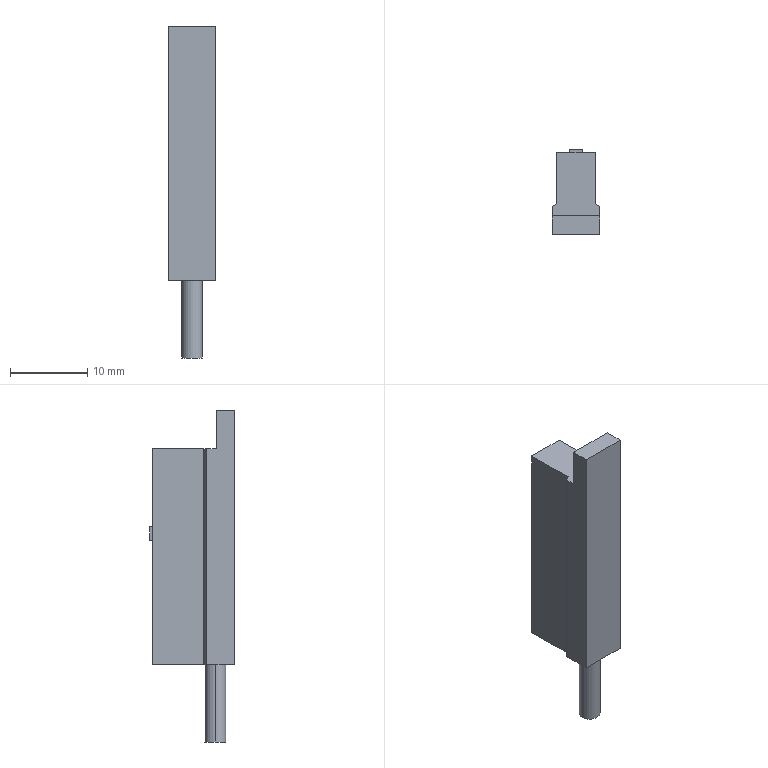Part | NX | 1 solid | 35 faces | box 6.2 x 10.996 x 43 mm | volume 1739 mm3 | plane 28 | cylinder 7 | commonest cylinder face diameters 2.347 x3 2.5 x2 2.7 x2
STEP:
#1=CARTESIAN_POINT('',(0.,2.35,-3.474));
#2=VERTEX_POINT('',#1);
#3=CARTESIAN_POINT('',(0.,1.35,-3.474));
#4=VERTEX_POINT('',#3);
#5=CARTESIAN_POINT('',(0.,2.35,-3.474));
#6=DIRECTION('',(0.,-1.,0.));
#7=VECTOR('',#6,1000.);
#8=LINE('',#5,#7);
#9=EDGE_CURVE('',#2,#4,#8,.T.);
#10=ORIENTED_EDGE('',*,*,#9,.F.);
#11=CARTESIAN_POINT('',(0.6555,2.35,-3.274));
#12=VERTEX_POINT('',#11);
#13=CARTESIAN_POINT('',(0.,2.35,-2.3));
#14=DIRECTION('',(0.,1.,0.));
#15=DIRECTION('',(0.,0.,1.));
#16=AXIS2_PLACEMENT_3D('',#13,#14,#15);
#17=CIRCLE('',#16,1.174);
#18=EDGE_CURVE('',#12,#2,#17,.T.);
#19=ORIENTED_EDGE('',*,*,#18,.F.);
#20=CARTESIAN_POINT('',(0.6555,1.35,-3.274));
#21=VERTEX_POINT('',#20);
#22=CARTESIAN_POINT('',(0.6555,2.35,-3.274));
#23=DIRECTION('',(0.,-1.,0.));
#24=VECTOR('',#23,1000.);
#25=LINE('',#22,#24);
#26=EDGE_CURVE('',#12,#21,#25,.T.);
#27=ORIENTED_EDGE('',*,*,#26,.T.);
#28=CARTESIAN_POINT('',(0.,1.35,-2.3));
#29=DIRECTION('',(0.,1.,0.));
#30=DIRECTION('',(0.,0.,1.));
#31=AXIS2_PLACEMENT_3D('',#28,#29,#30);
#32=CIRCLE('',#31,1.174);
#33=EDGE_CURVE('',#21,#4,#32,.T.);
#34=ORIENTED_EDGE('',*,*,#33,.T.);
#35=EDGE_LOOP('',(#10,#19,#27,#34));
#36=FACE_BOUND('',#35,.T.);
#37=CARTESIAN_POINT('',(0.,2.35,-2.3));
#38=DIRECTION('',(0.,-1.,0.));
#39=DIRECTION('',(0.,0.,-1.));
#40=AXIS2_PLACEMENT_3D('',#37,#38,#39);
#41=CYLINDRICAL_SURFACE('',#40,1.174);
#42=ADVANCED_FACE('',(#36),#41,.T.);
#43=CARTESIAN_POINT('',(0.,2.35,-1.05));
#44=VERTEX_POINT('',#43);
#45=CARTESIAN_POINT('',(0.,2.35,-3.55));
#46=VERTEX_POINT('',#45);
#47=CARTESIAN_POINT('',(0.,2.35,-2.3));
#48=DIRECTION('',(0.,-1.,0.));
#49=DIRECTION('',(0.,0.,-1.));
#50=AXIS2_PLACEMENT_3D('',#47,#48,#49);
#51=CIRCLE('',#50,1.25);
#52=EDGE_CURVE('',#44,#46,#51,.T.);
#53=ORIENTED_EDGE('',*,*,#52,.F.);
#54=CARTESIAN_POINT('',(0.,1.35,-1.05));
#55=VERTEX_POINT('',#54);
#56=CARTESIAN_POINT('',(0.,1.35,-1.05));
#57=DIRECTION('',(0.,1.,0.));
#58=VECTOR('',#57,1000.);
#59=LINE('',#56,#58);
#60=EDGE_CURVE('',#55,#44,#59,.T.);
#61=ORIENTED_EDGE('',*,*,#60,.F.);
#62=CARTESIAN_POINT('',(0.,1.35,-3.55));
#63=VERTEX_POINT('',#62);
#64=CARTESIAN_POINT('',(0.,1.35,-2.3));
#65=DIRECTION('',(0.,-1.,0.));
#66=DIRECTION('',(0.,0.,-1.));
#67=AXIS2_PLACEMENT_3D('',#64,#65,#66);
#68=CIRCLE('',#67,1.25);
#69=EDGE_CURVE('',#55,#63,#68,.T.);
#70=ORIENTED_EDGE('',*,*,#69,.T.);
#71=CARTESIAN_POINT('',(0.,1.35,-3.55));
#72=DIRECTION('',(0.,1.,0.));
#73=VECTOR('',#72,1000.);
#74=LINE('',#71,#73);
#75=EDGE_CURVE('',#63,#46,#74,.T.);
#76=ORIENTED_EDGE('',*,*,#75,.T.);
#77=EDGE_LOOP('',(#53,#61,#70,#76));
#78=FACE_BOUND('',#77,.T.);
#79=CARTESIAN_POINT('',(0.,1.35,-2.3));
#80=DIRECTION('',(0.,1.,0.));
#81=DIRECTION('',(0.,0.,1.));
#82=AXIS2_PLACEMENT_3D('',#79,#80,#81);
#83=CYLINDRICAL_SURFACE('',#82,1.25);
#84=ADVANCED_FACE('',(#78),#83,.F.);
#85=CARTESIAN_POINT('',(-1.35,2.496,-33.));
#86=VERTEX_POINT('',#85);
#87=CARTESIAN_POINT('',(1.35,2.496,-33.));
#88=VERTEX_POINT('',#87);
#89=CARTESIAN_POINT('',(0.,2.496,-33.));
#90=DIRECTION('',(0.,0.,-1.));
#91=DIRECTION('',(1.,0.,0.));
#92=AXIS2_PLACEMENT_3D('',#89,#90,#91);
#93=CIRCLE('',#92,1.35);
#94=EDGE_CURVE('',#86,#88,#93,.T.);
#95=ORIENTED_EDGE('',*,*,#94,.T.);
#96=CARTESIAN_POINT('',(1.35,2.496,-43.));
#97=VERTEX_POINT('',#96);
#98=CARTESIAN_POINT('',(1.35,2.496,-43.));
#99=DIRECTION('',(0.,0.,1.));
#100=VECTOR('',#99,1000.);
#101=LINE('',#98,#100);
#102=EDGE_CURVE('',#97,#88,#101,.T.);
#103=ORIENTED_EDGE('',*,*,#102,.F.);
#104=CARTESIAN_POINT('',(-1.35,2.496,-43.));
#105=VERTEX_POINT('',#104);
#106=CARTESIAN_POINT('',(0.,2.496,-43.));
#107=DIRECTION('',(0.,0.,-1.));
#108=DIRECTION('',(-1.,0.,0.));
#109=AXIS2_PLACEMENT_3D('',#106,#107,#108);
#110=CIRCLE('',#109,1.35);
#111=EDGE_CURVE('',#105,#97,#110,.T.);
#112=ORIENTED_EDGE('',*,*,#111,.F.);
#113=CARTESIAN_POINT('',(-1.35,2.496,-43.));
#114=DIRECTION('',(0.,0.,1.));
#115=VECTOR('',#114,1000.);
#116=LINE('',#113,#115);
#117=EDGE_CURVE('',#105,#86,#116,.T.);
#118=ORIENTED_EDGE('',*,*,#117,.T.);
#119=EDGE_LOOP('',(#95,#103,#112,#118));
#120=FACE_BOUND('',#119,.T.);
#121=CARTESIAN_POINT('',(0.,2.496,-43.));
#122=DIRECTION('',(0.,0.,1.));
#123=DIRECTION('',(1.,0.,0.));
#124=AXIS2_PLACEMENT_3D('',#121,#122,#123);
#125=CYLINDRICAL_SURFACE('',#124,1.35);
#126=ADVANCED_FACE('',(#120),#125,.T.);
#127=CARTESIAN_POINT('',(0.,1.35,-2.3));
#128=DIRECTION('',(0.,-1.,0.));
#129=DIRECTION('',(0.,0.,-1.));
#130=AXIS2_PLACEMENT_3D('',#127,#128,#129);
#131=CIRCLE('',#130,1.25);
#132=EDGE_CURVE('',#63,#55,#131,.T.);
#133=ORIENTED_EDGE('',*,*,#132,.F.);
#134=ORIENTED_EDGE('',*,*,#69,.F.);
#135=EDGE_LOOP('',(#133,#134));
#136=FACE_BOUND('',#135,.T.);
#137=ORIENTED_EDGE('',*,*,#33,.F.);
#138=CARTESIAN_POINT('',(-0.9737,1.35,-1.645));
#139=VERTEX_POINT('',#138);
#140=CARTESIAN_POINT('',(0.6555,1.35,-3.274));
#141=DIRECTION('',(0.7071,0.,-0.7071));
#142=VECTOR('',#141,1000.);
#143=LINE('',#140,#142);
#144=EDGE_CURVE('',#139,#21,#143,.T.);
#145=ORIENTED_EDGE('',*,*,#144,.F.);
#146=CARTESIAN_POINT('',(0.,1.35,-2.3));
#147=DIRECTION('',(0.,1.,0.));
#148=DIRECTION('',(0.,0.,1.));
#149=AXIS2_PLACEMENT_3D('',#146,#147,#148);
#150=CIRCLE('',#149,1.174);
#151=EDGE_CURVE('',#4,#139,#150,.T.);
#152=ORIENTED_EDGE('',*,*,#151,.F.);
#153=EDGE_LOOP('',(#137,#145,#152));
#154=FACE_BOUND('',#153,.T.);
#155=CARTESIAN_POINT('',(-0.647,1.35,-1.321));
#156=VERTEX_POINT('',#155);
#157=CARTESIAN_POINT('',(0.9793,1.35,-2.947));
#158=VERTEX_POINT('',#157);
#159=CARTESIAN_POINT('',(0.,1.35,-2.3));
#160=DIRECTION('',(0.,1.,0.));
#161=DIRECTION('',(0.,0.,1.));
#162=AXIS2_PLACEMENT_3D('',#159,#160,#161);
#163=CIRCLE('',#162,1.174);
#164=EDGE_CURVE('',#156,#158,#163,.T.);
#165=ORIENTED_EDGE('',*,*,#164,.F.);
#166=CARTESIAN_POINT('',(-0.647,1.35,-1.321));
#167=DIRECTION('',(-0.7071,0.,0.7071));
#168=VECTOR('',#167,1000.);
#169=LINE('',#166,#168);
#170=EDGE_CURVE('',#158,#156,#169,.T.);
#171=ORIENTED_EDGE('',*,*,#170,.F.);
#172=EDGE_LOOP('',(#165,#171));
#173=FACE_BOUND('',#172,.T.);
#174=CARTESIAN_POINT('',(0.,1.35,-2.3));
#175=DIRECTION('',(0.,-1.,0.));
#176=DIRECTION('',(0.,0.,-1.));
#177=AXIS2_PLACEMENT_3D('',#174,#175,#176);
#178=PLANE('',#177);
#179=ADVANCED_FACE('',(#136,#154,#173),#178,.F.);
#180=CARTESIAN_POINT('',(-3.1,2.35,0.));
#181=VERTEX_POINT('',#180);
#182=CARTESIAN_POINT('',(-3.1,2.35,-5.));
#183=VERTEX_POINT('',#182);
#184=CARTESIAN_POINT('',(-3.1,2.35,-5.));
#185=DIRECTION('',(0.,0.,-1.));
#186=VECTOR('',#185,1000.);
#187=LINE('',#184,#186);
#188=EDGE_CURVE('',#181,#183,#187,.T.);
#189=ORIENTED_EDGE('',*,*,#188,.F.);
#190=CARTESIAN_POINT('',(3.1,2.35,0.));
#191=VERTEX_POINT('',#190);
#192=CARTESIAN_POINT('',(-3.1,2.35,0.));
#193=DIRECTION('',(-1.,0.,0.));
#194=VECTOR('',#193,1000.);
#195=LINE('',#192,#194);
#196=EDGE_CURVE('',#191,#181,#195,.T.);
#197=ORIENTED_EDGE('',*,*,#196,.F.);
#198=CARTESIAN_POINT('',(3.1,2.35,-5.));
#199=VERTEX_POINT('',#198);
#200=CARTESIAN_POINT('',(3.1,2.35,0.));
#201=DIRECTION('',(0.,0.,1.));
#202=VECTOR('',#201,1000.);
#203=LINE('',#200,#202);
#204=EDGE_CURVE('',#199,#191,#203,.T.);
#205=ORIENTED_EDGE('',*,*,#204,.F.);
#206=CARTESIAN_POINT('',(3.1,2.35,-5.));
#207=DIRECTION('',(1.,0.,0.));
#208=VECTOR('',#207,1000.);
#209=LINE('',#206,#208);
#210=EDGE_CURVE('',#183,#199,#209,.T.);
#211=ORIENTED_EDGE('',*,*,#210,.F.);
#212=EDGE_LOOP('',(#189,#197,#205,#211));
#213=FACE_BOUND('',#212,.T.);
#214=ORIENTED_EDGE('',*,*,#52,.T.);
#215=CARTESIAN_POINT('',(0.,2.35,-2.3));
#216=DIRECTION('',(0.,-1.,0.));
#217=DIRECTION('',(0.,0.,-1.));
#218=AXIS2_PLACEMENT_3D('',#215,#216,#217);
#219=CIRCLE('',#218,1.25);
#220=EDGE_CURVE('',#46,#44,#219,.T.);
#221=ORIENTED_EDGE('',*,*,#220,.T.);
#222=EDGE_LOOP('',(#214,#221));
#223=FACE_BOUND('',#222,.T.);
#224=CARTESIAN_POINT('',(-3.1,2.35,0.));
#225=DIRECTION('',(0.,1.,0.));
#226=DIRECTION('',(1.,0.,0.));
#227=AXIS2_PLACEMENT_3D('',#224,#225,#226);
#228=PLANE('',#227);
#229=ADVANCED_FACE('',(#213,#223),#228,.T.);
#230=CARTESIAN_POINT('',(3.1,0.,0.));
#231=VERTEX_POINT('',#230);
#232=CARTESIAN_POINT('',(3.1,0.,0.));
#233=DIRECTION('',(0.,1.,0.));
#234=VECTOR('',#233,1000.);
#235=LINE('',#232,#234);
#236=EDGE_CURVE('',#231,#191,#235,.T.);
#237=ORIENTED_EDGE('',*,*,#236,.T.);
#238=ORIENTED_EDGE('',*,*,#196,.T.);
#239=CARTESIAN_POINT('',(-3.1,0.,0.));
#240=VERTEX_POINT('',#239);
#241=CARTESIAN_POINT('',(-3.1,0.,0.));
#242=DIRECTION('',(0.,-1.,0.));
#243=VECTOR('',#242,1000.);
#244=LINE('',#241,#243);
#245=EDGE_CURVE('',#181,#240,#244,.T.);
#246=ORIENTED_EDGE('',*,*,#245,.T.);
#247=CARTESIAN_POINT('',(-3.1,0.,0.));
#248=DIRECTION('',(1.,0.,0.));
#249=VECTOR('',#248,1000.);
#250=LINE('',#247,#249);
#251=EDGE_CURVE('',#240,#231,#250,.T.);
#252=ORIENTED_EDGE('',*,*,#251,.T.);
#253=EDGE_LOOP('',(#237,#238,#246,#252));
#254=FACE_BOUND('',#253,.T.);
#255=CARTESIAN_POINT('',(3.1,10.596,0.));
#256=DIRECTION('',(0.,0.,1.));
#257=DIRECTION('',(1.,0.,0.));
#258=AXIS2_PLACEMENT_3D('',#255,#256,#257);
#259=PLANE('',#258);
#260=ADVANCED_FACE('',(#254),#259,.T.);
#261=CARTESIAN_POINT('',(-1.,10.096,-17.));
#262=VERTEX_POINT('',#261);
#263=CARTESIAN_POINT('',(-1.,10.096,-15.));
#264=VERTEX_POINT('',#263);
#265=CARTESIAN_POINT('',(-1.,10.096,-15.));
#266=DIRECTION('',(0.,0.,1.));
#267=VECTOR('',#266,1000.);
#268=LINE('',#265,#267);
#269=EDGE_CURVE('',#262,#264,#268,.T.);
#270=ORIENTED_EDGE('',*,*,#269,.T.);
#271=CARTESIAN_POINT('',(1.,10.096,-15.));
#272=VERTEX_POINT('',#271);
#273=CARTESIAN_POINT('',(-1.,10.096,-15.));
#274=DIRECTION('',(1.,0.,0.));
#275=VECTOR('',#274,1000.);
#276=LINE('',#273,#275);
#277=EDGE_CURVE('',#264,#272,#276,.T.);
#278=ORIENTED_EDGE('',*,*,#277,.T.);
#279=CARTESIAN_POINT('',(1.,10.096,-17.));
#280=VERTEX_POINT('',#279);
#281=CARTESIAN_POINT('',(1.,10.096,-15.));
#282=DIRECTION('',(0.,0.,-1.));
#283=VECTOR('',#282,1000.);
#284=LINE('',#281,#283);
#285=EDGE_CURVE('',#272,#280,#284,.T.);
#286=ORIENTED_EDGE('',*,*,#285,.T.);
#287=CARTESIAN_POINT('',(-1.,10.096,-17.));
#288=DIRECTION('',(-1.,0.,0.));
#289=VECTOR('',#288,1000.);
#290=LINE('',#287,#289);
#291=EDGE_CURVE('',#280,#262,#290,.T.);
#292=ORIENTED_EDGE('',*,*,#291,.T.);
#293=EDGE_LOOP('',(#270,#278,#286,#292));
#294=FACE_BOUND('',#293,.T.);
#295=CARTESIAN_POINT('',(-0.875,10.096,-16.875));
#296=VERTEX_POINT('',#295);
#297=CARTESIAN_POINT('',(-0.875,10.096,-15.125));
#298=VERTEX_POINT('',#297);
#299=CARTESIAN_POINT('',(-0.875,10.096,-16.875));
#300=DIRECTION('',(0.,0.,1.));
#301=VECTOR('',#300,1000.);
#302=LINE('',#299,#301);
#303=EDGE_CURVE('',#296,#298,#302,.T.);
#304=ORIENTED_EDGE('',*,*,#303,.F.);
#305=CARTESIAN_POINT('',(0.875,10.096,-16.875));
#306=VERTEX_POINT('',#305);
#307=CARTESIAN_POINT('',(-0.875,10.096,-16.875));
#308=DIRECTION('',(-1.,0.,0.));
#309=VECTOR('',#308,1000.);
#310=LINE('',#307,#309);
#311=EDGE_CURVE('',#306,#296,#310,.T.);
#312=ORIENTED_EDGE('',*,*,#311,.F.);
#313=CARTESIAN_POINT('',(0.875,10.096,-15.125));
#314=VERTEX_POINT('',#313);
#315=CARTESIAN_POINT('',(0.875,10.096,-16.875));
#316=DIRECTION('',(0.,0.,-1.));
#317=VECTOR('',#316,1000.);
#318=LINE('',#315,#317);
#319=EDGE_CURVE('',#314,#306,#318,.T.);
#320=ORIENTED_EDGE('',*,*,#319,.F.);
#321=CARTESIAN_POINT('',(-0.875,10.096,-15.125));
#322=DIRECTION('',(1.,0.,0.));
#323=VECTOR('',#322,1000.);
#324=LINE('',#321,#323);
#325=EDGE_CURVE('',#298,#314,#324,.T.);
#326=ORIENTED_EDGE('',*,*,#325,.F.);
#327=EDGE_LOOP('',(#304,#312,#320,#326));
#328=FACE_BOUND('',#327,.T.);
#329=CARTESIAN_POINT('',(-1.,10.096,-17.));
#330=DIRECTION('',(0.,-1.,0.));
#331=DIRECTION('',(0.,0.,-1.));
#332=AXIS2_PLACEMENT_3D('',#329,#330,#331);
#333=PLANE('',#332);
#334=ADVANCED_FACE('',(#294,#328),#333,.F.);
#335=CARTESIAN_POINT('',(3.1,0.,-33.));
#336=VERTEX_POINT('',#335);
#337=CARTESIAN_POINT('',(3.1,3.6,-33.));
#338=VERTEX_POINT('',#337);
#339=CARTESIAN_POINT('',(3.1,0.,-33.));
#340=DIRECTION('',(0.,1.,0.));
#341=VECTOR('',#340,1000.);
#342=LINE('',#339,#341);
#343=EDGE_CURVE('',#336,#338,#342,.T.);
#344=ORIENTED_EDGE('',*,*,#343,.F.);
#345=CARTESIAN_POINT('',(-3.1,0.,-33.));
#346=VERTEX_POINT('',#345);
#347=CARTESIAN_POINT('',(-3.1,0.,-33.));
#348=DIRECTION('',(1.,0.,0.));
#349=VECTOR('',#348,1000.);
#350=LINE('',#347,#349);
#351=EDGE_CURVE('',#346,#336,#350,.T.);
#352=ORIENTED_EDGE('',*,*,#351,.F.);
#353=CARTESIAN_POINT('',(-3.1,3.6,-33.));
#354=VERTEX_POINT('',#353);
#355=CARTESIAN_POINT('',(-3.1,0.,-33.));
#356=DIRECTION('',(0.,-1.,0.));
#357=VECTOR('',#356,1000.);
#358=LINE('',#355,#357);
#359=EDGE_CURVE('',#354,#346,#358,.T.);
#360=ORIENTED_EDGE('',*,*,#359,.F.);
#361=CARTESIAN_POINT('',(-2.5,3.946,-33.));
#362=VERTEX_POINT('',#361);
#363=CARTESIAN_POINT('',(-3.1,3.6,-33.));
#364=DIRECTION('',(-0.866,-0.5,0.));
#365=VECTOR('',#364,1000.);
#366=LINE('',#363,#365);
#367=EDGE_CURVE('',#362,#354,#366,.T.);
#368=ORIENTED_EDGE('',*,*,#367,.F.);
#369=CARTESIAN_POINT('',(-2.5,10.596,-33.));
#370=VERTEX_POINT('',#369);
#371=CARTESIAN_POINT('',(-2.5,3.946,-33.));
#372=DIRECTION('',(0.,-1.,0.));
#373=VECTOR('',#372,1000.);
#374=LINE('',#371,#373);
#375=EDGE_CURVE('',#370,#362,#374,.T.);
#376=ORIENTED_EDGE('',*,*,#375,.F.);
#377=CARTESIAN_POINT('',(2.5,10.596,-33.));
#378=VERTEX_POINT('',#377);
#379=CARTESIAN_POINT('',(2.5,10.596,-33.));
#380=DIRECTION('',(-1.,0.,0.));
#381=VECTOR('',#380,1000.);
#382=LINE('',#379,#381);
#383=EDGE_CURVE('',#378,#370,#382,.T.);
#384=ORIENTED_EDGE('',*,*,#383,.F.);
#385=CARTESIAN_POINT('',(2.5,3.946,-33.));
#386=VERTEX_POINT('',#385);
#387=CARTESIAN_POINT('',(2.5,3.946,-33.));
#388=DIRECTION('',(0.,1.,0.));
#389=VECTOR('',#388,1000.);
#390=LINE('',#387,#389);
#391=EDGE_CURVE('',#386,#378,#390,.T.);
#392=ORIENTED_EDGE('',*,*,#391,.F.);
#393=CARTESIAN_POINT('',(3.1,3.6,-33.));
#394=DIRECTION('',(-0.866,0.5,0.));
#395=VECTOR('',#394,1000.);
#396=LINE('',#393,#395);
#397=EDGE_CURVE('',#338,#386,#396,.T.);
#398=ORIENTED_EDGE('',*,*,#397,.F.);
#399=EDGE_LOOP('',(#344,#352,#360,#368,#376,#384,#392,#398));
#400=FACE_BOUND('',#399,.T.);
#401=ORIENTED_EDGE('',*,*,#94,.F.);
#402=CARTESIAN_POINT('',(0.,2.496,-33.));
#403=DIRECTION('',(0.,0.,-1.));
#404=DIRECTION('',(1.,0.,0.));
#405=AXIS2_PLACEMENT_3D('',#402,#403,#404);
#406=CIRCLE('',#405,1.35);
#407=EDGE_CURVE('',#88,#86,#406,.T.);
#408=ORIENTED_EDGE('',*,*,#407,.F.);
#409=EDGE_LOOP('',(#401,#408));
#410=FACE_BOUND('',#409,.T.);
#411=CARTESIAN_POINT('',(3.1,10.596,-33.));
#412=DIRECTION('',(0.,0.,1.));
#413=DIRECTION('',(1.,0.,0.));
#414=AXIS2_PLACEMENT_3D('',#411,#412,#413);
#415=PLANE('',#414);
#416=ADVANCED_FACE('',(#400,#410),#415,.F.);
#417=CARTESIAN_POINT('',(3.1,3.6,-5.));
#418=VERTEX_POINT('',#417);
#419=CARTESIAN_POINT('',(3.1,10.996,-5.));
#420=DIRECTION('',(0.,-1.,0.));
#421=VECTOR('',#420,1000.);
#422=LINE('',#419,#421);
#423=EDGE_CURVE('',#418,#199,#422,.T.);
#424=ORIENTED_EDGE('',*,*,#423,.T.);
#425=ORIENTED_EDGE('',*,*,#204,.T.);
#426=ORIENTED_EDGE('',*,*,#236,.F.);
#427=CARTESIAN_POINT('',(3.1,0.,-33.));
#428=DIRECTION('',(0.,0.,1.));
#429=VECTOR('',#428,1000.);
#430=LINE('',#427,#429);
#431=EDGE_CURVE('',#336,#231,#430,.T.);
#432=ORIENTED_EDGE('',*,*,#431,.F.);
#433=ORIENTED_EDGE('',*,*,#343,.T.);
#434=CARTESIAN_POINT('',(3.1,3.6,-33.));
#435=DIRECTION('',(0.,0.,1.));
#436=VECTOR('',#435,1000.);
#437=LINE('',#434,#436);
#438=EDGE_CURVE('',#338,#418,#437,.T.);
#439=ORIENTED_EDGE('',*,*,#438,.T.);
#440=EDGE_LOOP('',(#424,#425,#426,#432,#433,#439));
#441=FACE_BOUND('',#440,.T.);
#442=CARTESIAN_POINT('',(3.1,0.,-33.));
#443=DIRECTION('',(1.,0.,0.));
#444=DIRECTION('',(0.,1.,0.));
#445=AXIS2_PLACEMENT_3D('',#442,#443,#444);
#446=PLANE('',#445);
#447=ADVANCED_FACE('',(#441),#446,.T.);
#448=ORIENTED_EDGE('',*,*,#251,.F.);
#449=CARTESIAN_POINT('',(-3.1,0.,-33.));
#450=DIRECTION('',(0.,0.,1.));
#451=VECTOR('',#450,1000.);
#452=LINE('',#449,#451);
#453=EDGE_CURVE('',#346,#240,#452,.T.);
#454=ORIENTED_EDGE('',*,*,#453,.F.);
#455=ORIENTED_EDGE('',*,*,#351,.T.);
#456=ORIENTED_EDGE('',*,*,#431,.T.);
#457=EDGE_LOOP('',(#448,#454,#455,#456));
#458=FACE_BOUND('',#457,.T.);
#459=CARTESIAN_POINT('',(-3.1,0.,-33.));
#460=DIRECTION('',(0.,-1.,0.));
#461=DIRECTION('',(0.,0.,-1.));
#462=AXIS2_PLACEMENT_3D('',#459,#460,#461);
#463=PLANE('',#462);
#464=ADVANCED_FACE('',(#458),#463,.T.);
#465=CARTESIAN_POINT('',(-3.1,3.6,-5.));
#466=VERTEX_POINT('',#465);
#467=CARTESIAN_POINT('',(-3.1,10.996,-5.));
#468=DIRECTION('',(0.,-1.,0.));
#469=VECTOR('',#468,1000.);
#470=LINE('',#467,#469);
#471=EDGE_CURVE('',#466,#183,#470,.T.);
#472=ORIENTED_EDGE('',*,*,#471,.F.);
#473=CARTESIAN_POINT('',(-3.1,3.6,-33.));
#474=DIRECTION('',(0.,0.,1.));
#475=VECTOR('',#474,1000.);
#476=LINE('',#473,#475);
#477=EDGE_CURVE('',#354,#466,#476,.T.);
#478=ORIENTED_EDGE('',*,*,#477,.F.);
#479=ORIENTED_EDGE('',*,*,#359,.T.);
#480=ORIENTED_EDGE('',*,*,#453,.T.);
#481=ORIENTED_EDGE('',*,*,#245,.F.);
#482=ORIENTED_EDGE('',*,*,#188,.T.);
#483=EDGE_LOOP('',(#472,#478,#479,#480,#481,#482));
#484=FACE_BOUND('',#483,.T.);
#485=CARTESIAN_POINT('',(-3.1,0.,-33.));
#486=DIRECTION('',(-1.,0.,0.));
#487=DIRECTION('',(0.,0.,1.));
#488=AXIS2_PLACEMENT_3D('',#485,#486,#487);
#489=PLANE('',#488);
#490=ADVANCED_FACE('',(#484),#489,.T.);
#491=CARTESIAN_POINT('',(-2.5,3.946,-5.));
#492=VERTEX_POINT('',#491);
#493=CARTESIAN_POINT('',(-3.1,3.6,-5.));
#494=DIRECTION('',(-0.866,-0.5,0.));
#495=VECTOR('',#494,1000.);
#496=LINE('',#493,#495);
#497=EDGE_CURVE('',#492,#466,#496,.T.);
#498=ORIENTED_EDGE('',*,*,#497,.F.);
#499=CARTESIAN_POINT('',(-2.5,3.946,-33.));
#500=DIRECTION('',(0.,0.,1.));
#501=VECTOR('',#500,1000.);
#502=LINE('',#499,#501);
#503=EDGE_CURVE('',#362,#492,#502,.T.);
#504=ORIENTED_EDGE('',*,*,#503,.F.);
#505=ORIENTED_EDGE('',*,*,#367,.T.);
#506=ORIENTED_EDGE('',*,*,#477,.T.);
#507=EDGE_LOOP('',(#498,#504,#505,#506));
#508=FACE_BOUND('',#507,.T.);
#509=CARTESIAN_POINT('',(-3.1,3.6,-33.));
#510=DIRECTION('',(-0.5,0.866,0.));
#511=DIRECTION('',(0.,0.,1.));
#512=AXIS2_PLACEMENT_3D('',#509,#510,#511);
#513=PLANE('',#512);
#514=ADVANCED_FACE('',(#508),#513,.T.);
#515=CARTESIAN_POINT('',(-2.5,10.596,-5.));
#516=VERTEX_POINT('',#515);
#517=CARTESIAN_POINT('',(-2.5,3.946,-5.));
#518=DIRECTION('',(0.,-1.,0.));
#519=VECTOR('',#518,1000.);
#520=LINE('',#517,#519);
#521=EDGE_CURVE('',#516,#492,#520,.T.);
#522=ORIENTED_EDGE('',*,*,#521,.F.);
#523=CARTESIAN_POINT('',(-2.5,10.596,-33.));
#524=DIRECTION('',(0.,0.,1.));
#525=VECTOR('',#524,1000.);
#526=LINE('',#523,#525);
#527=EDGE_CURVE('',#370,#516,#526,.T.);
#528=ORIENTED_EDGE('',*,*,#527,.F.);
#529=ORIENTED_EDGE('',*,*,#375,.T.);
#530=ORIENTED_EDGE('',*,*,#503,.T.);
#531=EDGE_LOOP('',(#522,#528,#529,#530));
#532=FACE_BOUND('',#531,.T.);
#533=CARTESIAN_POINT('',(-2.5,3.946,-33.));
#534=DIRECTION('',(-1.,0.,0.));
#535=DIRECTION('',(0.,0.,1.));
#536=AXIS2_PLACEMENT_3D('',#533,#534,#535);
#537=PLANE('',#536);
#538=ADVANCED_FACE('',(#532),#537,.T.);
#539=CARTESIAN_POINT('',(2.5,10.596,-5.));
#540=VERTEX_POINT('',#539);
#541=CARTESIAN_POINT('',(2.5,10.596,-5.));
#542=DIRECTION('',(-1.,0.,0.));
#543=VECTOR('',#542,1000.);
#544=LINE('',#541,#543);
#545=EDGE_CURVE('',#540,#516,#544,.T.);
#546=ORIENTED_EDGE('',*,*,#545,.F.);
#547=CARTESIAN_POINT('',(2.5,10.596,-33.));
#548=DIRECTION('',(0.,0.,1.));
#549=VECTOR('',#548,1000.);
#550=LINE('',#547,#549);
#551=EDGE_CURVE('',#378,#540,#550,.T.);
#552=ORIENTED_EDGE('',*,*,#551,.F.);
#553=ORIENTED_EDGE('',*,*,#383,.T.);
#554=ORIENTED_EDGE('',*,*,#527,.T.);
#555=EDGE_LOOP('',(#546,#552,#553,#554));
#556=FACE_BOUND('',#555,.T.);
#557=CARTESIAN_POINT('',(-1.,10.596,-17.));
#558=VERTEX_POINT('',#557);
#559=CARTESIAN_POINT('',(-1.,10.596,-15.));
#560=VERTEX_POINT('',#559);
#561=CARTESIAN_POINT('',(-1.,10.596,-15.));
#562=DIRECTION('',(0.,0.,1.));
#563=VECTOR('',#562,1000.);
#564=LINE('',#561,#563);
#565=EDGE_CURVE('',#558,#560,#564,.T.);
#566=ORIENTED_EDGE('',*,*,#565,.F.);
#567=CARTESIAN_POINT('',(1.,10.596,-17.));
#568=VERTEX_POINT('',#567);
#569=CARTESIAN_POINT('',(-1.,10.596,-17.));
#570=DIRECTION('',(-1.,0.,0.));
#571=VECTOR('',#570,1000.);
#572=LINE('',#569,#571);
#573=EDGE_CURVE('',#568,#558,#572,.T.);
#574=ORIENTED_EDGE('',*,*,#573,.F.);
#575=CARTESIAN_POINT('',(1.,10.596,-15.));
#576=VERTEX_POINT('',#575);
#577=CARTESIAN_POINT('',(1.,10.596,-15.));
#578=DIRECTION('',(0.,0.,-1.));
#579=VECTOR('',#578,1000.);
#580=LINE('',#577,#579);
#581=EDGE_CURVE('',#576,#568,#580,.T.);
#582=ORIENTED_EDGE('',*,*,#581,.F.);
#583=CARTESIAN_POINT('',(-1.,10.596,-15.));
#584=DIRECTION('',(1.,0.,0.));
#585=VECTOR('',#584,1000.);
#586=LINE('',#583,#585);
#587=EDGE_CURVE('',#560,#576,#586,.T.);
#588=ORIENTED_EDGE('',*,*,#587,.F.);
#589=EDGE_LOOP('',(#566,#574,#582,#588));
#590=FACE_BOUND('',#589,.T.);
#591=CARTESIAN_POINT('',(2.5,10.596,-33.));
#592=DIRECTION('',(0.,1.,0.));
#593=DIRECTION('',(1.,0.,0.));
#594=AXIS2_PLACEMENT_3D('',#591,#592,#593);
#595=PLANE('',#594);
#596=ADVANCED_FACE('',(#556,#590),#595,.T.);
#597=CARTESIAN_POINT('',(2.5,3.946,-5.));
#598=VERTEX_POINT('',#597);
#599=CARTESIAN_POINT('',(2.5,3.946,-5.));
#600=DIRECTION('',(0.,1.,0.));
#601=VECTOR('',#600,1000.);
#602=LINE('',#599,#601);
#603=EDGE_CURVE('',#598,#540,#602,.T.);
#604=ORIENTED_EDGE('',*,*,#603,.F.);
#605=CARTESIAN_POINT('',(2.5,3.946,-33.));
#606=DIRECTION('',(0.,0.,1.));
#607=VECTOR('',#606,1000.);
#608=LINE('',#605,#607);
#609=EDGE_CURVE('',#386,#598,#608,.T.);
#610=ORIENTED_EDGE('',*,*,#609,.F.);
#611=ORIENTED_EDGE('',*,*,#391,.T.);
#612=ORIENTED_EDGE('',*,*,#551,.T.);
#613=EDGE_LOOP('',(#604,#610,#611,#612));
#614=FACE_BOUND('',#613,.T.);
#615=CARTESIAN_POINT('',(2.5,3.946,-33.));
#616=DIRECTION('',(1.,0.,0.));
#617=DIRECTION('',(0.,-1.,0.));
#618=AXIS2_PLACEMENT_3D('',#615,#616,#617);
#619=PLANE('',#618);
#620=ADVANCED_FACE('',(#614),#619,.T.);
#621=CARTESIAN_POINT('',(3.1,3.6,-5.));
#622=DIRECTION('',(-0.866,0.5,0.));
#623=VECTOR('',#622,1000.);
#624=LINE('',#621,#623);
#625=EDGE_CURVE('',#418,#598,#624,.T.);
#626=ORIENTED_EDGE('',*,*,#625,.F.);
#627=ORIENTED_EDGE('',*,*,#438,.F.);
#628=ORIENTED_EDGE('',*,*,#397,.T.);
#629=ORIENTED_EDGE('',*,*,#609,.T.);
#630=EDGE_LOOP('',(#626,#627,#628,#629));
#631=FACE_BOUND('',#630,.T.);
#632=CARTESIAN_POINT('',(3.1,3.6,-33.));
#633=DIRECTION('',(0.5,0.866,0.));
#634=DIRECTION('',(0.,0.,-1.));
#635=AXIS2_PLACEMENT_3D('',#632,#633,#634);
#636=PLANE('',#635);
#637=ADVANCED_FACE('',(#631),#636,.T.);
#638=ORIENTED_EDGE('',*,*,#164,.T.);
#639=CARTESIAN_POINT('',(0.9793,2.35,-2.947));
#640=VERTEX_POINT('',#639);
#641=CARTESIAN_POINT('',(0.9793,2.35,-2.947));
#642=DIRECTION('',(0.,-1.,0.));
#643=VECTOR('',#642,1000.);
#644=LINE('',#641,#643);
#645=EDGE_CURVE('',#158,#640,#644,.F.);
#646=ORIENTED_EDGE('',*,*,#645,.T.);
#647=CARTESIAN_POINT('',(-0.647,2.35,-1.321));
#648=VERTEX_POINT('',#647);
#649=CARTESIAN_POINT('',(0.,2.35,-2.3));
#650=DIRECTION('',(0.,1.,0.));
#651=DIRECTION('',(0.,0.,1.));
#652=AXIS2_PLACEMENT_3D('',#649,#650,#651);
#653=CIRCLE('',#652,1.174);
#654=EDGE_CURVE('',#648,#640,#653,.T.);
#655=ORIENTED_EDGE('',*,*,#654,.F.);
#656=CARTESIAN_POINT('',(-0.647,2.35,-1.321));
#657=DIRECTION('',(0.,-1.,0.));
#658=VECTOR('',#657,1000.);
#659=LINE('',#656,#658);
#660=EDGE_CURVE('',#156,#648,#659,.F.);
#661=ORIENTED_EDGE('',*,*,#660,.F.);
#662=EDGE_LOOP('',(#638,#646,#655,#661));
#663=FACE_BOUND('',#662,.T.);
#664=CARTESIAN_POINT('',(0.,2.35,-2.3));
#665=DIRECTION('',(0.,-1.,0.));
#666=DIRECTION('',(0.,0.,-1.));
#667=AXIS2_PLACEMENT_3D('',#664,#665,#666);
#668=CYLINDRICAL_SURFACE('',#667,1.174);
#669=ADVANCED_FACE('',(#663),#668,.T.);
#670=CARTESIAN_POINT('',(0.,2.496,-43.));
#671=DIRECTION('',(0.,0.,-1.));
#672=DIRECTION('',(-1.,0.,0.));
#673=AXIS2_PLACEMENT_3D('',#670,#671,#672);
#674=CIRCLE('',#673,1.35);
#675=EDGE_CURVE('',#97,#105,#674,.T.);
#676=ORIENTED_EDGE('',*,*,#675,.T.);
#677=ORIENTED_EDGE('',*,*,#111,.T.);
#678=EDGE_LOOP('',(#676,#677));
#679=FACE_BOUND('',#678,.T.);
#680=CARTESIAN_POINT('',(0.,2.496,-43.));
#681=DIRECTION('',(0.,0.,-1.));
#682=DIRECTION('',(0.,-1.,0.));
#683=AXIS2_PLACEMENT_3D('',#680,#681,#682);
#684=PLANE('',#683);
#685=ADVANCED_FACE('',(#679),#684,.T.);
#686=ORIENTED_EDGE('',*,*,#565,.T.);
#687=CARTESIAN_POINT('',(-1.,10.096,-15.));
#688=DIRECTION('',(0.,1.,0.));
#689=VECTOR('',#688,1000.);
#690=LINE('',#687,#689);
#691=EDGE_CURVE('',#264,#560,#690,.T.);
#692=ORIENTED_EDGE('',*,*,#691,.F.);
#693=ORIENTED_EDGE('',*,*,#269,.F.);
#694=CARTESIAN_POINT('',(-1.,10.096,-17.));
#695=DIRECTION('',(0.,1.,0.));
#696=VECTOR('',#695,1000.);
#697=LINE('',#694,#696);
#698=EDGE_CURVE('',#262,#558,#697,.T.);
#699=ORIENTED_EDGE('',*,*,#698,.T.);
#700=EDGE_LOOP('',(#686,#692,#693,#699));
#701=FACE_BOUND('',#700,.T.);
#702=CARTESIAN_POINT('',(-1.,10.096,-15.));
#703=DIRECTION('',(-1.,0.,0.));
#704=DIRECTION('',(0.,1.,0.));
#705=AXIS2_PLACEMENT_3D('',#702,#703,#704);
#706=PLANE('',#705);
#707=ADVANCED_FACE('',(#701),#706,.F.);
#708=ORIENTED_EDGE('',*,*,#573,.T.);
#709=ORIENTED_EDGE('',*,*,#698,.F.);
#710=ORIENTED_EDGE('',*,*,#291,.F.);
#711=CARTESIAN_POINT('',(1.,10.096,-17.));
#712=DIRECTION('',(0.,1.,0.));
#713=VECTOR('',#712,1000.);
#714=LINE('',#711,#713);
#715=EDGE_CURVE('',#280,#568,#714,.T.);
#716=ORIENTED_EDGE('',*,*,#715,.T.);
#717=EDGE_LOOP('',(#708,#709,#710,#716));
#718=FACE_BOUND('',#717,.T.);
#719=CARTESIAN_POINT('',(-1.,10.096,-17.));
#720=DIRECTION('',(0.,0.,-1.));
#721=DIRECTION('',(0.,-1.,0.));
#722=AXIS2_PLACEMENT_3D('',#719,#720,#721);
#723=PLANE('',#722);
#724=ADVANCED_FACE('',(#718),#723,.F.);
#725=ORIENTED_EDGE('',*,*,#581,.T.);
#726=ORIENTED_EDGE('',*,*,#715,.F.);
#727=ORIENTED_EDGE('',*,*,#285,.F.);
#728=CARTESIAN_POINT('',(1.,10.096,-15.));
#729=DIRECTION('',(0.,1.,0.));
#730=VECTOR('',#729,1000.);
#731=LINE('',#728,#730);
#732=EDGE_CURVE('',#272,#576,#731,.T.);
#733=ORIENTED_EDGE('',*,*,#732,.T.);
#734=EDGE_LOOP('',(#725,#726,#727,#733));
#735=FACE_BOUND('',#734,.T.);
#736=CARTESIAN_POINT('',(1.,10.096,-15.));
#737=DIRECTION('',(1.,0.,0.));
#738=DIRECTION('',(0.,0.,-1.));
#739=AXIS2_PLACEMENT_3D('',#736,#737,#738);
#740=PLANE('',#739);
#741=ADVANCED_FACE('',(#735),#740,.F.);
#742=ORIENTED_EDGE('',*,*,#587,.T.);
#743=ORIENTED_EDGE('',*,*,#732,.F.);
#744=ORIENTED_EDGE('',*,*,#277,.F.);
#745=ORIENTED_EDGE('',*,*,#691,.T.);
#746=EDGE_LOOP('',(#742,#743,#744,#745));
#747=FACE_BOUND('',#746,.T.);
#748=CARTESIAN_POINT('',(-1.,10.096,-15.));
#749=DIRECTION('',(0.,0.,1.));
#750=DIRECTION('',(1.,0.,0.));
#751=AXIS2_PLACEMENT_3D('',#748,#749,#750);
#752=PLANE('',#751);
#753=ADVANCED_FACE('',(#747),#752,.F.);
#754=ORIENTED_EDGE('',*,*,#303,.T.);
#755=CARTESIAN_POINT('',(-0.875,10.996,-15.125));
#756=VERTEX_POINT('',#755);
#757=CARTESIAN_POINT('',(-0.875,10.996,-15.125));
#758=DIRECTION('',(0.,-1.,0.));
#759=VECTOR('',#758,1000.);
#760=LINE('',#757,#759);
#761=EDGE_CURVE('',#756,#298,#760,.T.);
#762=ORIENTED_EDGE('',*,*,#761,.F.);
#763=CARTESIAN_POINT('',(-0.875,10.996,-16.875));
#764=VERTEX_POINT('',#763);
#765=CARTESIAN_POINT('',(-0.875,10.996,-16.875));
#766=DIRECTION('',(0.,0.,1.));
#767=VECTOR('',#766,1000.);
#768=LINE('',#765,#767);
#769=EDGE_CURVE('',#764,#756,#768,.T.);
#770=ORIENTED_EDGE('',*,*,#769,.F.);
#771=CARTESIAN_POINT('',(-0.875,10.996,-16.875));
#772=DIRECTION('',(0.,-1.,0.));
#773=VECTOR('',#772,1000.);
#774=LINE('',#771,#773);
#775=EDGE_CURVE('',#764,#296,#774,.T.);
#776=ORIENTED_EDGE('',*,*,#775,.T.);
#777=EDGE_LOOP('',(#754,#762,#770,#776));
#778=FACE_BOUND('',#777,.T.);
#779=CARTESIAN_POINT('',(-0.875,10.996,-16.875));
#780=DIRECTION('',(1.,0.,0.));
#781=DIRECTION('',(0.,0.,-1.));
#782=AXIS2_PLACEMENT_3D('',#779,#780,#781);
#783=PLANE('',#782);
#784=ADVANCED_FACE('',(#778),#783,.F.);
#785=ORIENTED_EDGE('',*,*,#325,.T.);
#786=CARTESIAN_POINT('',(0.875,10.996,-15.125));
#787=VERTEX_POINT('',#786);
#788=CARTESIAN_POINT('',(0.875,10.996,-15.125));
#789=DIRECTION('',(0.,-1.,0.));
#790=VECTOR('',#789,1000.);
#791=LINE('',#788,#790);
#792=EDGE_CURVE('',#787,#314,#791,.T.);
#793=ORIENTED_EDGE('',*,*,#792,.F.);
#794=CARTESIAN_POINT('',(-0.875,10.996,-15.125));
#795=DIRECTION('',(1.,0.,0.));
#796=VECTOR('',#795,1000.);
#797=LINE('',#794,#796);
#798=EDGE_CURVE('',#756,#787,#797,.T.);
#799=ORIENTED_EDGE('',*,*,#798,.F.);
#800=ORIENTED_EDGE('',*,*,#761,.T.);
#801=EDGE_LOOP('',(#785,#793,#799,#800));
#802=FACE_BOUND('',#801,.T.);
#803=CARTESIAN_POINT('',(-0.875,10.996,-15.125));
#804=DIRECTION('',(0.,0.,-1.));
#805=DIRECTION('',(-1.,0.,0.));
#806=AXIS2_PLACEMENT_3D('',#803,#804,#805);
#807=PLANE('',#806);
#808=ADVANCED_FACE('',(#802),#807,.F.);
#809=ORIENTED_EDGE('',*,*,#319,.T.);
#810=CARTESIAN_POINT('',(0.875,10.996,-16.875));
#811=VERTEX_POINT('',#810);
#812=CARTESIAN_POINT('',(0.875,10.996,-16.875));
#813=DIRECTION('',(0.,-1.,0.));
#814=VECTOR('',#813,1000.);
#815=LINE('',#812,#814);
#816=EDGE_CURVE('',#811,#306,#815,.T.);
#817=ORIENTED_EDGE('',*,*,#816,.F.);
#818=CARTESIAN_POINT('',(0.875,10.996,-16.875));
#819=DIRECTION('',(0.,0.,-1.));
#820=VECTOR('',#819,1000.);
#821=LINE('',#818,#820);
#822=EDGE_CURVE('',#787,#811,#821,.T.);
#823=ORIENTED_EDGE('',*,*,#822,.F.);
#824=ORIENTED_EDGE('',*,*,#792,.T.);
#825=EDGE_LOOP('',(#809,#817,#823,#824));
#826=FACE_BOUND('',#825,.T.);
#827=CARTESIAN_POINT('',(0.875,10.996,-16.875));
#828=DIRECTION('',(-1.,0.,0.));
#829=DIRECTION('',(0.,1.,0.));
#830=AXIS2_PLACEMENT_3D('',#827,#828,#829);
#831=PLANE('',#830);
#832=ADVANCED_FACE('',(#826),#831,.F.);
#833=ORIENTED_EDGE('',*,*,#311,.T.);
#834=ORIENTED_EDGE('',*,*,#775,.F.);
#835=CARTESIAN_POINT('',(-0.875,10.996,-16.875));
#836=DIRECTION('',(-1.,0.,0.));
#837=VECTOR('',#836,1000.);
#838=LINE('',#835,#837);
#839=EDGE_CURVE('',#811,#764,#838,.T.);
#840=ORIENTED_EDGE('',*,*,#839,.F.);
#841=ORIENTED_EDGE('',*,*,#816,.T.);
#842=EDGE_LOOP('',(#833,#834,#840,#841));
#843=FACE_BOUND('',#842,.T.);
#844=CARTESIAN_POINT('',(-0.875,10.996,-16.875));
#845=DIRECTION('',(0.,0.,1.));
#846=DIRECTION('',(1.,0.,0.));
#847=AXIS2_PLACEMENT_3D('',#844,#845,#846);
#848=PLANE('',#847);
#849=ADVANCED_FACE('',(#843),#848,.F.);
#850=ORIENTED_EDGE('',*,*,#769,.T.);
#851=ORIENTED_EDGE('',*,*,#798,.T.);
#852=ORIENTED_EDGE('',*,*,#822,.T.);
#853=ORIENTED_EDGE('',*,*,#839,.T.);
#854=EDGE_LOOP('',(#850,#851,#852,#853));
#855=FACE_BOUND('',#854,.T.);
#856=CARTESIAN_POINT('',(-0.875,10.996,-16.875));
#857=DIRECTION('',(0.,1.,0.));
#858=DIRECTION('',(1.,0.,0.));
#859=AXIS2_PLACEMENT_3D('',#856,#857,#858);
#860=PLANE('',#859);
#861=ADVANCED_FACE('',(#855),#860,.T.);
#862=ORIENTED_EDGE('',*,*,#497,.T.);
#863=ORIENTED_EDGE('',*,*,#471,.T.);
#864=ORIENTED_EDGE('',*,*,#210,.T.);
#865=ORIENTED_EDGE('',*,*,#423,.F.);
#866=ORIENTED_EDGE('',*,*,#625,.T.);
#867=ORIENTED_EDGE('',*,*,#603,.T.);
#868=ORIENTED_EDGE('',*,*,#545,.T.);
#869=ORIENTED_EDGE('',*,*,#521,.T.);
#870=EDGE_LOOP('',(#862,#863,#864,#865,#866,#867,#868,#869));
#871=FACE_BOUND('',#870,.T.);
#872=CARTESIAN_POINT('',(3.1,10.996,-5.));
#873=DIRECTION('',(0.,0.,-1.));
#874=DIRECTION('',(0.,-1.,0.));
#875=AXIS2_PLACEMENT_3D('',#872,#873,#874);
#876=PLANE('',#875);
#877=ADVANCED_FACE('',(#871),#876,.F.);
#878=ORIENTED_EDGE('',*,*,#170,.T.);
#879=ORIENTED_EDGE('',*,*,#660,.T.);
#880=CARTESIAN_POINT('',(-0.647,2.35,-1.321));
#881=DIRECTION('',(-0.7071,0.,0.7071));
#882=VECTOR('',#881,1000.);
#883=LINE('',#880,#882);
#884=EDGE_CURVE('',#640,#648,#883,.T.);
#885=ORIENTED_EDGE('',*,*,#884,.F.);
#886=ORIENTED_EDGE('',*,*,#645,.F.);
#887=EDGE_LOOP('',(#878,#879,#885,#886));
#888=FACE_BOUND('',#887,.T.);
#889=CARTESIAN_POINT('',(-0.647,2.35,-1.321));
#890=DIRECTION('',(0.7071,0.,0.7071));
#891=DIRECTION('',(0.,-1.,0.));
#892=AXIS2_PLACEMENT_3D('',#889,#890,#891);
#893=PLANE('',#892);
#894=ADVANCED_FACE('',(#888),#893,.F.);
#895=ORIENTED_EDGE('',*,*,#654,.T.);
#896=ORIENTED_EDGE('',*,*,#884,.T.);
#897=EDGE_LOOP('',(#895,#896));
#898=FACE_BOUND('',#897,.T.);
#899=CARTESIAN_POINT('',(0.,2.35,-2.3));
#900=DIRECTION('',(0.,1.,0.));
#901=DIRECTION('',(1.,0.,0.));
#902=AXIS2_PLACEMENT_3D('',#899,#900,#901);
#903=PLANE('',#902);
#904=ADVANCED_FACE('',(#898),#903,.T.);
#905=ORIENTED_EDGE('',*,*,#144,.T.);
#906=ORIENTED_EDGE('',*,*,#26,.F.);
#907=CARTESIAN_POINT('',(-0.9737,2.35,-1.645));
#908=VERTEX_POINT('',#907);
#909=CARTESIAN_POINT('',(0.6555,2.35,-3.274));
#910=DIRECTION('',(0.7071,0.,-0.7071));
#911=VECTOR('',#910,1000.);
#912=LINE('',#909,#911);
#913=EDGE_CURVE('',#908,#12,#912,.T.);
#914=ORIENTED_EDGE('',*,*,#913,.F.);
#915=CARTESIAN_POINT('',(-0.9737,2.35,-1.645));
#916=DIRECTION('',(0.,-1.,0.));
#917=VECTOR('',#916,1000.);
#918=LINE('',#915,#917);
#919=EDGE_CURVE('',#908,#139,#918,.T.);
#920=ORIENTED_EDGE('',*,*,#919,.T.);
#921=EDGE_LOOP('',(#905,#906,#914,#920));
#922=FACE_BOUND('',#921,.T.);
#923=CARTESIAN_POINT('',(0.6555,2.35,-3.274));
#924=DIRECTION('',(-0.7071,0.,-0.7071));
#925=DIRECTION('',(-0.7071,0.,0.7071));
#926=AXIS2_PLACEMENT_3D('',#923,#924,#925);
#927=PLANE('',#926);
#928=ADVANCED_FACE('',(#922),#927,.F.);
#929=ORIENTED_EDGE('',*,*,#18,.T.);
#930=CARTESIAN_POINT('',(0.,2.35,-2.3));
#931=DIRECTION('',(0.,1.,0.));
#932=DIRECTION('',(0.,0.,1.));
#933=AXIS2_PLACEMENT_3D('',#930,#931,#932);
#934=CIRCLE('',#933,1.174);
#935=EDGE_CURVE('',#2,#908,#934,.T.);
#936=ORIENTED_EDGE('',*,*,#935,.T.);
#937=ORIENTED_EDGE('',*,*,#913,.T.);
#938=EDGE_LOOP('',(#929,#936,#937));
#939=FACE_BOUND('',#938,.T.);
#940=CARTESIAN_POINT('',(0.,2.35,-2.3));
#941=DIRECTION('',(0.,1.,0.));
#942=DIRECTION('',(1.,0.,0.));
#943=AXIS2_PLACEMENT_3D('',#940,#941,#942);
#944=PLANE('',#943);
#945=ADVANCED_FACE('',(#939),#944,.T.);
#946=ORIENTED_EDGE('',*,*,#132,.T.);
#947=ORIENTED_EDGE('',*,*,#60,.T.);
#948=ORIENTED_EDGE('',*,*,#220,.F.);
#949=ORIENTED_EDGE('',*,*,#75,.F.);
#950=EDGE_LOOP('',(#946,#947,#948,#949));
#951=FACE_BOUND('',#950,.T.);
#952=CARTESIAN_POINT('',(0.,1.35,-2.3));
#953=DIRECTION('',(0.,1.,0.));
#954=DIRECTION('',(0.,0.,1.));
#955=AXIS2_PLACEMENT_3D('',#952,#953,#954);
#956=CYLINDRICAL_SURFACE('',#955,1.25);
#957=ADVANCED_FACE('',(#951),#956,.F.);
#958=ORIENTED_EDGE('',*,*,#675,.F.);
#959=ORIENTED_EDGE('',*,*,#102,.T.);
#960=ORIENTED_EDGE('',*,*,#407,.T.);
#961=ORIENTED_EDGE('',*,*,#117,.F.);
#962=EDGE_LOOP('',(#958,#959,#960,#961));
#963=FACE_BOUND('',#962,.T.);
#964=CARTESIAN_POINT('',(0.,2.496,-43.));
#965=DIRECTION('',(0.,0.,1.));
#966=DIRECTION('',(1.,0.,0.));
#967=AXIS2_PLACEMENT_3D('',#964,#965,#966);
#968=CYLINDRICAL_SURFACE('',#967,1.35);
#969=ADVANCED_FACE('',(#963),#968,.T.);
#970=ORIENTED_EDGE('',*,*,#935,.F.);
#971=ORIENTED_EDGE('',*,*,#9,.T.);
#972=ORIENTED_EDGE('',*,*,#151,.T.);
#973=ORIENTED_EDGE('',*,*,#919,.F.);
#974=EDGE_LOOP('',(#970,#971,#972,#973));
#975=FACE_BOUND('',#974,.T.);
#976=CARTESIAN_POINT('',(0.,2.35,-2.3));
#977=DIRECTION('',(0.,-1.,0.));
#978=DIRECTION('',(0.,0.,-1.));
#979=AXIS2_PLACEMENT_3D('',#976,#977,#978);
#980=CYLINDRICAL_SURFACE('',#979,1.174);
#981=ADVANCED_FACE('',(#975),#980,.T.);
#982=CLOSED_SHELL('',(#42,#84,#126,#179,#229,#260,#334,#416,#447,#464,#490,#514,#538,#596,#620,#637,#669,#685,#707,#724,#741,#753,#784,#808,#832,#849,#861,#877,#894,#904,#928,#945,#957,#969,#981));
#983=MANIFOLD_SOLID_BREP('',#982);
#984=(LENGTH_UNIT()NAMED_UNIT(*)SI_UNIT(.MILLI.,.METRE.));
#985=UNCERTAINTY_MEASURE_WITH_UNIT(LENGTH_MEASURE(0.00001),#984,'','');
#986=(NAMED_UNIT(*)PLANE_ANGLE_UNIT()SI_UNIT($,.RADIAN.));
#987=(NAMED_UNIT(*)SI_UNIT($,.STERADIAN.)SOLID_ANGLE_UNIT());
#988=(GEOMETRIC_REPRESENTATION_CONTEXT(3)GLOBAL_UNCERTAINTY_ASSIGNED_CONTEXT((#985))GLOBAL_UNIT_ASSIGNED_CONTEXT((#984,#986,#987))REPRESENTATION_CONTEXT('',''));
#989=ADVANCED_BREP_SHAPE_REPRESENTATION('',(#983),#988);